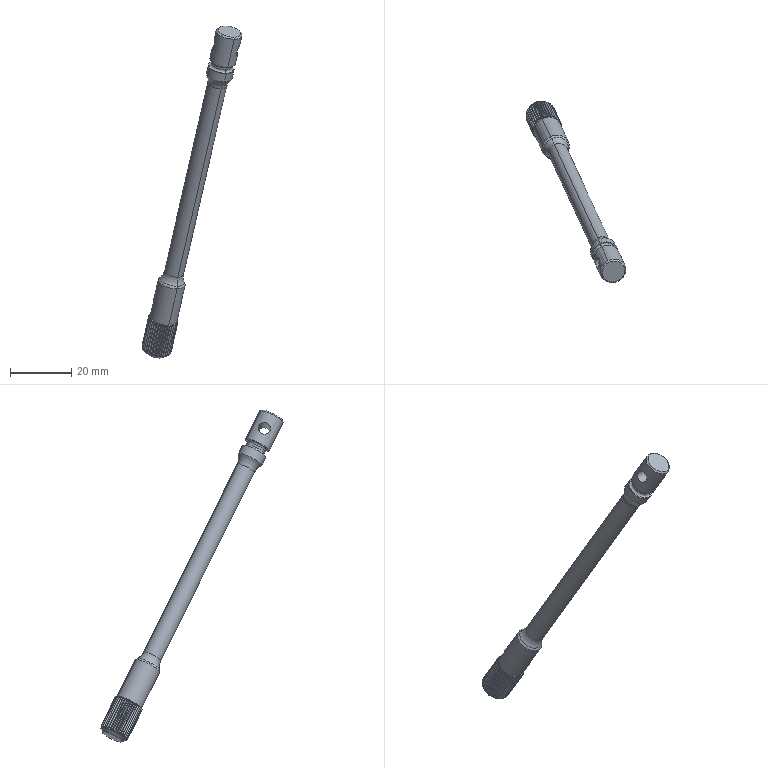Part | SolidWorks | features BaseBody 1 | 1 solid | 246 faces | box 32.722 x 59.616 x 108.746 mm | volume 4991 mm3 | plane 142 | cone 49 | cylinder 47 | torus 8 | commonest cylinder face diameters 0.16 x35 8.605 x4 3.983 x2 6.3 x2 6.6 x2 9 x2